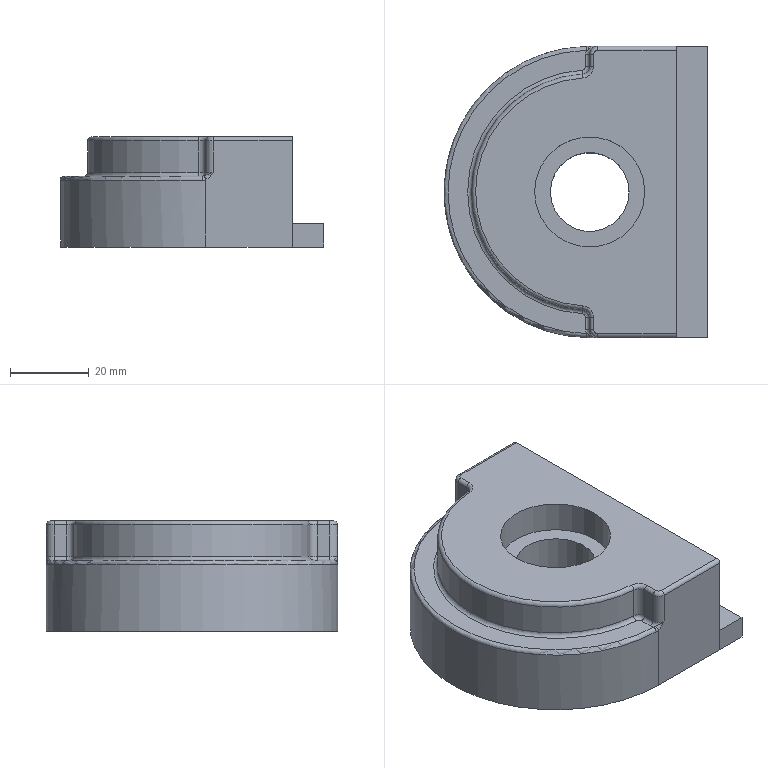Part | NX | features DATUM_CSYS 6, SKETCH 5, HOLE PACKAGE 3, BLEND 2, EXTRUDE 2, MIRROR_SET 2, SIMPLE HOLE 2, THREADS 2, CBORE_HOLE 1, SKIN 1 | 2 solids | 58 faces | box 67 x 74 x 28 mm | volume 88703 mm3 | plane 19 | cylinder 18 | torus 11 | spline 10 | commonest cylinder face diameters 2 x6 4 x4 8.5 x2 10 x2 20 x1 28 x1